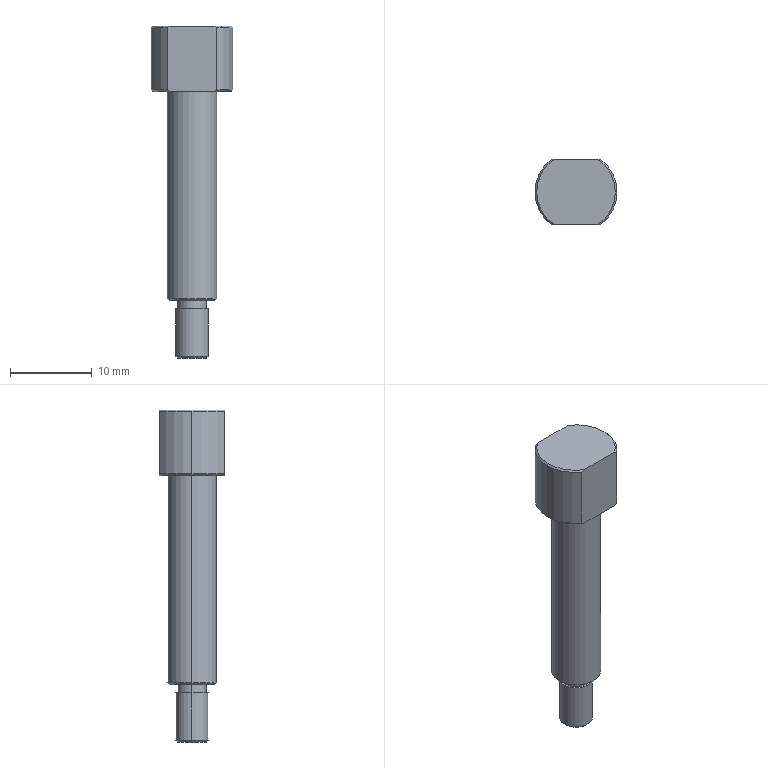Part | SolidWorks | features ICE 4, Chamfer 3, Extrusion 1 | 1 solid | 26 faces | box 10 x 8 x 40.5 mm | volume 1368 mm3 | cone 10 | cylinder 9 | plane 7 | commonest cylinder face diameters 10 x3 3.5 x2 4 x2 6 x2
STEP:
#1=CARTESIAN_POINT('',(2.,0.,-19.55));
#2=VERTEX_POINT('',#1);
#3=CARTESIAN_POINT('',(-2.,0.,-19.55));
#4=VERTEX_POINT('',#3);
#5=CARTESIAN_POINT('',(0.,0.,-19.55));
#6=DIRECTION('',(0.,0.,1.));
#7=DIRECTION('',(-1.,0.,0.));
#8=AXIS2_PLACEMENT_3D('',#5,#6,#7);
#9=CIRCLE('',#8,2.);
#10=EDGE_CURVE('',#2,#4,#9,.T.);
#11=ORIENTED_EDGE('',*,*,#10,.T.);
#12=CARTESIAN_POINT('',(-2.,0.,-13.75));
#13=VERTEX_POINT('',#12);
#14=CARTESIAN_POINT('',(-2.,0.,-19.75));
#15=DIRECTION('',(0.,0.,1.));
#16=VECTOR('',#15,1000.);
#17=LINE('',#14,#16);
#18=EDGE_CURVE('',#4,#13,#17,.T.);
#19=ORIENTED_EDGE('',*,*,#18,.T.);
#20=CARTESIAN_POINT('',(2.,0.,-13.75));
#21=VERTEX_POINT('',#20);
#22=CARTESIAN_POINT('',(0.,0.,-13.75));
#23=DIRECTION('',(0.,0.,-1.));
#24=DIRECTION('',(-1.,0.,0.));
#25=AXIS2_PLACEMENT_3D('',#22,#23,#24);
#26=CIRCLE('',#25,2.);
#27=EDGE_CURVE('',#13,#21,#26,.T.);
#28=ORIENTED_EDGE('',*,*,#27,.T.);
#29=CARTESIAN_POINT('',(2.,0.,-19.75));
#30=DIRECTION('',(0.,0.,1.));
#31=VECTOR('',#30,1000.);
#32=LINE('',#29,#31);
#33=EDGE_CURVE('',#2,#21,#32,.T.);
#34=ORIENTED_EDGE('',*,*,#33,.F.);
#35=EDGE_LOOP('',(#11,#19,#28,#34));
#36=FACE_OUTER_BOUND('',#35,.T.);
#37=CARTESIAN_POINT('',(0.,0.,-19.75));
#38=DIRECTION('',(0.,0.,1.));
#39=DIRECTION('',(1.,0.,0.));
#40=AXIS2_PLACEMENT_3D('',#37,#38,#39);
#41=CYLINDRICAL_SURFACE('',#40,2.);
#42=ADVANCED_FACE('',(#36),#41,.T.);
#43=CARTESIAN_POINT('',(-1.8,0.,-19.75));
#44=VERTEX_POINT('',#43);
#45=CARTESIAN_POINT('',(1.8,0.,-19.75));
#46=VERTEX_POINT('',#45);
#47=CARTESIAN_POINT('',(0.,0.,-19.75));
#48=DIRECTION('',(0.,0.,-1.));
#49=DIRECTION('',(-1.,0.,0.));
#50=AXIS2_PLACEMENT_3D('',#47,#48,#49);
#51=CIRCLE('',#50,1.8);
#52=EDGE_CURVE('',#44,#46,#51,.T.);
#53=ORIENTED_EDGE('',*,*,#52,.F.);
#54=CARTESIAN_POINT('',(-1.8,0.,-19.75));
#55=DIRECTION('',(-0.7071,0.,0.7071));
#56=VECTOR('',#55,1000.);
#57=LINE('',#54,#56);
#58=EDGE_CURVE('',#44,#4,#57,.T.);
#59=ORIENTED_EDGE('',*,*,#58,.T.);
#60=ORIENTED_EDGE('',*,*,#10,.F.);
#61=CARTESIAN_POINT('',(1.8,0.,-19.75));
#62=DIRECTION('',(0.7071,0.,0.7071));
#63=VECTOR('',#62,1000.);
#64=LINE('',#61,#63);
#65=EDGE_CURVE('',#46,#2,#64,.T.);
#66=ORIENTED_EDGE('',*,*,#65,.F.);
#67=EDGE_LOOP('',(#53,#59,#60,#66));
#68=FACE_OUTER_BOUND('',#67,.T.);
#69=CARTESIAN_POINT('',(0.,0.,-19.75));
#70=DIRECTION('',(0.,0.,1.));
#71=DIRECTION('',(1.,0.,0.));
#72=AXIS2_PLACEMENT_3D('',#69,#70,#71);
#73=CONICAL_SURFACE('',#72,1.8,0.7854);
#74=ADVANCED_FACE('',(#68),#73,.T.);
#75=CARTESIAN_POINT('',(-1.75,0.,-13.75));
#76=VERTEX_POINT('',#75);
#77=CARTESIAN_POINT('',(1.75,0.,-13.75));
#78=VERTEX_POINT('',#77);
#79=CARTESIAN_POINT('',(0.,0.,-13.75));
#80=DIRECTION('',(0.,0.,-1.));
#81=DIRECTION('',(-1.,0.,0.));
#82=AXIS2_PLACEMENT_3D('',#79,#80,#81);
#83=CIRCLE('',#82,1.75);
#84=EDGE_CURVE('',#76,#78,#83,.T.);
#85=ORIENTED_EDGE('',*,*,#84,.F.);
#86=CARTESIAN_POINT('',(-1.75,0.,-12.75));
#87=VERTEX_POINT('',#86);
#88=CARTESIAN_POINT('',(-1.75,0.,-13.75));
#89=DIRECTION('',(0.,0.,1.));
#90=VECTOR('',#89,1000.);
#91=LINE('',#88,#90);
#92=EDGE_CURVE('',#76,#87,#91,.T.);
#93=ORIENTED_EDGE('',*,*,#92,.T.);
#94=CARTESIAN_POINT('',(1.75,0.,-12.75));
#95=VERTEX_POINT('',#94);
#96=CARTESIAN_POINT('',(0.,0.,-12.75));
#97=DIRECTION('',(0.,0.,-1.));
#98=DIRECTION('',(-1.,0.,0.));
#99=AXIS2_PLACEMENT_3D('',#96,#97,#98);
#100=CIRCLE('',#99,1.75);
#101=EDGE_CURVE('',#87,#95,#100,.T.);
#102=ORIENTED_EDGE('',*,*,#101,.T.);
#103=CARTESIAN_POINT('',(1.75,0.,-13.75));
#104=DIRECTION('',(0.,0.,1.));
#105=VECTOR('',#104,1000.);
#106=LINE('',#103,#105);
#107=EDGE_CURVE('',#78,#95,#106,.T.);
#108=ORIENTED_EDGE('',*,*,#107,.F.);
#109=EDGE_LOOP('',(#85,#93,#102,#108));
#110=FACE_OUTER_BOUND('',#109,.T.);
#111=CARTESIAN_POINT('',(0.,0.,-13.75));
#112=DIRECTION('',(0.,0.,1.));
#113=DIRECTION('',(1.,0.,0.));
#114=AXIS2_PLACEMENT_3D('',#111,#112,#113);
#115=CYLINDRICAL_SURFACE('',#114,1.75);
#116=ADVANCED_FACE('',(#110),#115,.T.);
#117=CARTESIAN_POINT('',(4.8,0.,12.75));
#118=VERTEX_POINT('',#117);
#119=CARTESIAN_POINT('',(2.653,-4.,12.75));
#120=VERTEX_POINT('',#119);
#121=CARTESIAN_POINT('',(0.,0.,12.75));
#122=DIRECTION('',(0.,0.,-1.));
#123=DIRECTION('',(1.,0.,0.));
#124=AXIS2_PLACEMENT_3D('',#121,#122,#123);
#125=CIRCLE('',#124,4.8);
#126=EDGE_CURVE('',#118,#120,#125,.T.);
#127=ORIENTED_EDGE('',*,*,#126,.F.);
#128=CARTESIAN_POINT('',(5.,0.,12.95));
#129=VERTEX_POINT('',#128);
#130=CARTESIAN_POINT('',(5.,0.,12.95));
#131=DIRECTION('',(0.7071,0.,0.7071));
#132=VECTOR('',#131,1000.);
#133=LINE('',#130,#132);
#134=EDGE_CURVE('',#118,#129,#133,.T.);
#135=ORIENTED_EDGE('',*,*,#134,.T.);
#136=CARTESIAN_POINT('',(3.,-4.,12.95));
#137=VERTEX_POINT('',#136);
#138=CARTESIAN_POINT('',(0.,0.,12.95));
#139=DIRECTION('',(0.,0.,1.));
#140=DIRECTION('',(1.,0.,0.));
#141=AXIS2_PLACEMENT_3D('',#138,#139,#140);
#142=CIRCLE('',#141,5.);
#143=EDGE_CURVE('',#137,#129,#142,.T.);
#144=ORIENTED_EDGE('',*,*,#143,.F.);
#145=CARTESIAN_POINT('',(2.653,-4.,12.75));
#146=CARTESIAN_POINT('',(2.77,-4.,12.815));
#147=CARTESIAN_POINT('',(2.886,-4.,12.881));
#148=CARTESIAN_POINT('',(3.,-4.,12.95));
#149=B_SPLINE_CURVE_WITH_KNOTS('',3,(#145,#146,#147,#148),.UNSPECIFIED.,.F.,.F.,(4,4),(0.01544,0.01584),.UNSPECIFIED.);
#150=EDGE_CURVE('',#120,#137,#149,.T.);
#151=ORIENTED_EDGE('',*,*,#150,.F.);
#152=EDGE_LOOP('',(#127,#135,#144,#151));
#153=FACE_OUTER_BOUND('',#152,.T.);
#154=CARTESIAN_POINT('',(0.,0.,12.95));
#155=DIRECTION('',(0.,0.,1.));
#156=DIRECTION('',(1.,0.,0.));
#157=AXIS2_PLACEMENT_3D('',#154,#155,#156);
#158=CONICAL_SURFACE('',#157,5.,0.7854);
#159=ADVANCED_FACE('',(#153),#158,.T.);
#160=CARTESIAN_POINT('',(-4.8,0.,20.75));
#161=VERTEX_POINT('',#160);
#162=CARTESIAN_POINT('',(-2.653,-4.,20.75));
#163=VERTEX_POINT('',#162);
#164=CARTESIAN_POINT('',(0.,0.,20.75));
#165=DIRECTION('',(0.,0.,1.));
#166=DIRECTION('',(1.,0.,0.));
#167=AXIS2_PLACEMENT_3D('',#164,#165,#166);
#168=CIRCLE('',#167,4.8);
#169=EDGE_CURVE('',#161,#163,#168,.T.);
#170=ORIENTED_EDGE('',*,*,#169,.F.);
#171=CARTESIAN_POINT('',(-5.,0.,20.55));
#172=VERTEX_POINT('',#171);
#173=CARTESIAN_POINT('',(-4.8,0.,20.75));
#174=DIRECTION('',(-0.7071,0.,-0.7071));
#175=VECTOR('',#174,1000.);
#176=LINE('',#173,#175);
#177=EDGE_CURVE('',#161,#172,#176,.T.);
#178=ORIENTED_EDGE('',*,*,#177,.T.);
#179=CARTESIAN_POINT('',(-3.,-4.,20.55));
#180=VERTEX_POINT('',#179);
#181=CARTESIAN_POINT('',(0.,0.,20.55));
#182=DIRECTION('',(0.,0.,-1.));
#183=DIRECTION('',(1.,0.,0.));
#184=AXIS2_PLACEMENT_3D('',#181,#182,#183);
#185=CIRCLE('',#184,5.);
#186=EDGE_CURVE('',#180,#172,#185,.T.);
#187=ORIENTED_EDGE('',*,*,#186,.F.);
#188=CARTESIAN_POINT('',(-2.653,-4.,20.75));
#189=CARTESIAN_POINT('',(-2.77,-4.,20.685));
#190=CARTESIAN_POINT('',(-2.886,-4.,20.619));
#191=CARTESIAN_POINT('',(-3.,-4.,20.55));
#192=B_SPLINE_CURVE_WITH_KNOTS('',3,(#188,#189,#190,#191),.UNSPECIFIED.,.F.,.F.,(4,4),(0.01544,0.01584),.UNSPECIFIED.);
#193=EDGE_CURVE('',#163,#180,#192,.T.);
#194=ORIENTED_EDGE('',*,*,#193,.F.);
#195=EDGE_LOOP('',(#170,#178,#187,#194));
#196=FACE_OUTER_BOUND('',#195,.T.);
#197=CARTESIAN_POINT('',(0.,0.,20.75));
#198=DIRECTION('',(0.,0.,-1.));
#199=DIRECTION('',(-1.,0.,0.));
#200=AXIS2_PLACEMENT_3D('',#197,#198,#199);
#201=CONICAL_SURFACE('',#200,4.8,0.7854);
#202=ADVANCED_FACE('',(#196),#201,.T.);
#203=ORIENTED_EDGE('',*,*,#186,.T.);
#204=CARTESIAN_POINT('',(-5.,0.,12.95));
#205=VERTEX_POINT('',#204);
#206=CARTESIAN_POINT('',(-5.,0.,20.75));
#207=DIRECTION('',(0.,0.,-1.));
#208=VECTOR('',#207,1000.);
#209=LINE('',#206,#208);
#210=EDGE_CURVE('',#172,#205,#209,.T.);
#211=ORIENTED_EDGE('',*,*,#210,.T.);
#212=CARTESIAN_POINT('',(-3.,-4.,12.95));
#213=VERTEX_POINT('',#212);
#214=CARTESIAN_POINT('',(0.,0.,12.95));
#215=DIRECTION('',(0.,0.,1.));
#216=DIRECTION('',(1.,0.,0.));
#217=AXIS2_PLACEMENT_3D('',#214,#215,#216);
#218=CIRCLE('',#217,5.);
#219=EDGE_CURVE('',#205,#213,#218,.T.);
#220=ORIENTED_EDGE('',*,*,#219,.T.);
#221=CARTESIAN_POINT('',(-3.,-4.,20.75));
#222=DIRECTION('',(0.,0.,1.));
#223=VECTOR('',#222,1000.);
#224=LINE('',#221,#223);
#225=EDGE_CURVE('',#213,#180,#224,.T.);
#226=ORIENTED_EDGE('',*,*,#225,.T.);
#227=EDGE_LOOP('',(#203,#211,#220,#226));
#228=FACE_OUTER_BOUND('',#227,.T.);
#229=CARTESIAN_POINT('',(0.,0.,20.75));
#230=DIRECTION('',(0.,0.,-1.));
#231=DIRECTION('',(-1.,0.,0.));
#232=AXIS2_PLACEMENT_3D('',#229,#230,#231);
#233=CYLINDRICAL_SURFACE('',#232,5.);
#234=ADVANCED_FACE('',(#228),#233,.T.);
#235=CARTESIAN_POINT('',(-2.8,0.,-12.75));
#236=VERTEX_POINT('',#235);
#237=CARTESIAN_POINT('',(2.8,0.,-12.75));
#238=VERTEX_POINT('',#237);
#239=CARTESIAN_POINT('',(0.,0.,-12.75));
#240=DIRECTION('',(0.,0.,-1.));
#241=DIRECTION('',(1.,0.,0.));
#242=AXIS2_PLACEMENT_3D('',#239,#240,#241);
#243=CIRCLE('',#242,2.8);
#244=EDGE_CURVE('',#236,#238,#243,.T.);
#245=ORIENTED_EDGE('',*,*,#244,.F.);
#246=CARTESIAN_POINT('',(-3.,0.,-12.55));
#247=VERTEX_POINT('',#246);
#248=CARTESIAN_POINT('',(-3.,0.,-12.55));
#249=DIRECTION('',(-0.7071,0.,0.7071));
#250=VECTOR('',#249,1000.);
#251=LINE('',#248,#250);
#252=EDGE_CURVE('',#236,#247,#251,.T.);
#253=ORIENTED_EDGE('',*,*,#252,.T.);
#254=CARTESIAN_POINT('',(3.,0.,-12.55));
#255=VERTEX_POINT('',#254);
#256=CARTESIAN_POINT('',(0.,0.,-12.55));
#257=DIRECTION('',(0.,0.,1.));
#258=DIRECTION('',(1.,0.,0.));
#259=AXIS2_PLACEMENT_3D('',#256,#257,#258);
#260=CIRCLE('',#259,3.);
#261=EDGE_CURVE('',#255,#247,#260,.T.);
#262=ORIENTED_EDGE('',*,*,#261,.F.);
#263=CARTESIAN_POINT('',(3.,0.,-12.55));
#264=DIRECTION('',(0.7071,0.,0.7071));
#265=VECTOR('',#264,1000.);
#266=LINE('',#263,#265);
#267=EDGE_CURVE('',#238,#255,#266,.T.);
#268=ORIENTED_EDGE('',*,*,#267,.F.);
#269=EDGE_LOOP('',(#245,#253,#262,#268));
#270=FACE_OUTER_BOUND('',#269,.T.);
#271=CARTESIAN_POINT('',(0.,0.,-12.55));
#272=DIRECTION('',(0.,0.,1.));
#273=DIRECTION('',(1.,0.,0.));
#274=AXIS2_PLACEMENT_3D('',#271,#272,#273);
#275=CONICAL_SURFACE('',#274,3.,0.7854);
#276=ADVANCED_FACE('',(#270),#275,.T.);
#277=CARTESIAN_POINT('',(3.,0.,12.75));
#278=VERTEX_POINT('',#277);
#279=CARTESIAN_POINT('',(-3.,0.,12.75));
#280=VERTEX_POINT('',#279);
#281=CARTESIAN_POINT('',(0.,0.,12.75));
#282=DIRECTION('',(0.,0.,1.));
#283=DIRECTION('',(1.,0.,0.));
#284=AXIS2_PLACEMENT_3D('',#281,#282,#283);
#285=CIRCLE('',#284,3.);
#286=EDGE_CURVE('',#278,#280,#285,.T.);
#287=ORIENTED_EDGE('',*,*,#286,.F.);
#288=CARTESIAN_POINT('',(3.,0.,12.75));
#289=DIRECTION('',(0.,0.,-1.));
#290=VECTOR('',#289,1000.);
#291=LINE('',#288,#290);
#292=EDGE_CURVE('',#278,#255,#291,.T.);
#293=ORIENTED_EDGE('',*,*,#292,.T.);
#294=ORIENTED_EDGE('',*,*,#261,.T.);
#295=CARTESIAN_POINT('',(-3.,0.,12.75));
#296=DIRECTION('',(0.,0.,-1.));
#297=VECTOR('',#296,1000.);
#298=LINE('',#295,#297);
#299=EDGE_CURVE('',#280,#247,#298,.T.);
#300=ORIENTED_EDGE('',*,*,#299,.F.);
#301=EDGE_LOOP('',(#287,#293,#294,#300));
#302=FACE_OUTER_BOUND('',#301,.T.);
#303=CARTESIAN_POINT('',(0.,0.,12.75));
#304=DIRECTION('',(0.,0.,-1.));
#305=DIRECTION('',(-1.,0.,0.));
#306=AXIS2_PLACEMENT_3D('',#303,#304,#305);
#307=CYLINDRICAL_SURFACE('',#306,3.);
#308=ADVANCED_FACE('',(#302),#307,.T.);
#309=CARTESIAN_POINT('',(3.,4.,20.55));
#310=VERTEX_POINT('',#309);
#311=CARTESIAN_POINT('',(3.,-4.,20.55));
#312=VERTEX_POINT('',#311);
#313=CARTESIAN_POINT('',(0.,0.,20.55));
#314=DIRECTION('',(0.,0.,-1.));
#315=DIRECTION('',(1.,0.,0.));
#316=AXIS2_PLACEMENT_3D('',#313,#314,#315);
#317=CIRCLE('',#316,5.);
#318=EDGE_CURVE('',#310,#312,#317,.T.);
#319=ORIENTED_EDGE('',*,*,#318,.T.);
#320=CARTESIAN_POINT('',(3.,-4.,20.75));
#321=DIRECTION('',(0.,0.,-1.));
#322=VECTOR('',#321,1000.);
#323=LINE('',#320,#322);
#324=EDGE_CURVE('',#312,#137,#323,.T.);
#325=ORIENTED_EDGE('',*,*,#324,.T.);
#326=ORIENTED_EDGE('',*,*,#143,.T.);
#327=CARTESIAN_POINT('',(3.,4.,12.95));
#328=VERTEX_POINT('',#327);
#329=CARTESIAN_POINT('',(0.,0.,12.95));
#330=DIRECTION('',(0.,0.,1.));
#331=DIRECTION('',(1.,0.,0.));
#332=AXIS2_PLACEMENT_3D('',#329,#330,#331);
#333=CIRCLE('',#332,5.);
#334=EDGE_CURVE('',#129,#328,#333,.T.);
#335=ORIENTED_EDGE('',*,*,#334,.T.);
#336=CARTESIAN_POINT('',(3.,4.,20.75));
#337=DIRECTION('',(0.,0.,1.));
#338=VECTOR('',#337,1000.);
#339=LINE('',#336,#338);
#340=EDGE_CURVE('',#328,#310,#339,.T.);
#341=ORIENTED_EDGE('',*,*,#340,.T.);
#342=EDGE_LOOP('',(#319,#325,#326,#335,#341));
#343=FACE_OUTER_BOUND('',#342,.T.);
#344=CARTESIAN_POINT('',(0.,0.,20.75));
#345=DIRECTION('',(0.,0.,-1.));
#346=DIRECTION('',(-1.,0.,0.));
#347=AXIS2_PLACEMENT_3D('',#344,#345,#346);
#348=CYLINDRICAL_SURFACE('',#347,5.);
#349=ADVANCED_FACE('',(#343),#348,.T.);
#350=CARTESIAN_POINT('',(2.653,-4.,20.75));
#351=VERTEX_POINT('',#350);
#352=CARTESIAN_POINT('',(3.,-4.,20.55));
#353=CARTESIAN_POINT('',(2.885,-4.,20.619));
#354=CARTESIAN_POINT('',(2.77,-4.,20.686));
#355=CARTESIAN_POINT('',(2.653,-4.,20.75));
#356=B_SPLINE_CURVE_WITH_KNOTS('',3,(#352,#353,#354,#355),.UNSPECIFIED.,.F.,.F.,(4,4),(0.009425,0.009825),.UNSPECIFIED.);
#357=EDGE_CURVE('',#312,#351,#356,.T.);
#358=ORIENTED_EDGE('',*,*,#357,.F.);
#359=ORIENTED_EDGE('',*,*,#318,.F.);
#360=CARTESIAN_POINT('',(2.653,4.,20.75));
#361=VERTEX_POINT('',#360);
#362=CARTESIAN_POINT('',(2.653,4.,20.75));
#363=CARTESIAN_POINT('',(2.77,4.,20.685));
#364=CARTESIAN_POINT('',(2.886,4.,20.619));
#365=CARTESIAN_POINT('',(3.,4.,20.55));
#366=B_SPLINE_CURVE_WITH_KNOTS('',3,(#362,#363,#364,#365),.UNSPECIFIED.,.F.,.F.,(4,4),(0.01544,0.01584),.UNSPECIFIED.);
#367=EDGE_CURVE('',#361,#310,#366,.T.);
#368=ORIENTED_EDGE('',*,*,#367,.F.);
#369=CARTESIAN_POINT('',(0.,0.,20.75));
#370=DIRECTION('',(0.,0.,1.));
#371=DIRECTION('',(1.,0.,0.));
#372=AXIS2_PLACEMENT_3D('',#369,#370,#371);
#373=CIRCLE('',#372,4.8);
#374=EDGE_CURVE('',#351,#361,#373,.T.);
#375=ORIENTED_EDGE('',*,*,#374,.F.);
#376=EDGE_LOOP('',(#358,#359,#368,#375));
#377=FACE_OUTER_BOUND('',#376,.T.);
#378=CARTESIAN_POINT('',(0.,0.,20.75));
#379=DIRECTION('',(0.,0.,-1.));
#380=DIRECTION('',(-1.,0.,0.));
#381=AXIS2_PLACEMENT_3D('',#378,#379,#380);
#382=CONICAL_SURFACE('',#381,4.8,0.7854);
#383=ADVANCED_FACE('',(#377),#382,.T.);
#384=CARTESIAN_POINT('',(-2.653,-4.,12.75));
#385=VERTEX_POINT('',#384);
#386=CARTESIAN_POINT('',(-3.,-4.,12.95));
#387=CARTESIAN_POINT('',(-2.885,-4.,12.881));
#388=CARTESIAN_POINT('',(-2.77,-4.,12.814));
#389=CARTESIAN_POINT('',(-2.653,-4.,12.75));
#390=B_SPLINE_CURVE_WITH_KNOTS('',3,(#386,#387,#388,#389),.UNSPECIFIED.,.F.,.F.,(4,4),(0.009425,0.009825),.UNSPECIFIED.);
#391=EDGE_CURVE('',#213,#385,#390,.T.);
#392=ORIENTED_EDGE('',*,*,#391,.F.);
#393=ORIENTED_EDGE('',*,*,#219,.F.);
#394=CARTESIAN_POINT('',(-3.,4.,12.95));
#395=VERTEX_POINT('',#394);
#396=CARTESIAN_POINT('',(0.,0.,12.95));
#397=DIRECTION('',(0.,0.,1.));
#398=DIRECTION('',(1.,0.,0.));
#399=AXIS2_PLACEMENT_3D('',#396,#397,#398);
#400=CIRCLE('',#399,5.);
#401=EDGE_CURVE('',#395,#205,#400,.T.);
#402=ORIENTED_EDGE('',*,*,#401,.F.);
#403=CARTESIAN_POINT('',(-2.653,4.,12.75));
#404=VERTEX_POINT('',#403);
#405=CARTESIAN_POINT('',(-2.653,4.,12.75));
#406=CARTESIAN_POINT('',(-2.77,4.,12.815));
#407=CARTESIAN_POINT('',(-2.886,4.,12.881));
#408=CARTESIAN_POINT('',(-3.,4.,12.95));
#409=B_SPLINE_CURVE_WITH_KNOTS('',3,(#405,#406,#407,#408),.UNSPECIFIED.,.F.,.F.,(4,4),(0.01544,0.01584),.UNSPECIFIED.);
#410=EDGE_CURVE('',#404,#395,#409,.T.);
#411=ORIENTED_EDGE('',*,*,#410,.F.);
#412=CARTESIAN_POINT('',(0.,0.,12.75));
#413=DIRECTION('',(0.,0.,-1.));
#414=DIRECTION('',(1.,0.,0.));
#415=AXIS2_PLACEMENT_3D('',#412,#413,#414);
#416=CIRCLE('',#415,4.8);
#417=EDGE_CURVE('',#385,#404,#416,.T.);
#418=ORIENTED_EDGE('',*,*,#417,.F.);
#419=EDGE_LOOP('',(#392,#393,#402,#411,#418));
#420=FACE_OUTER_BOUND('',#419,.T.);
#421=CARTESIAN_POINT('',(0.,0.,12.95));
#422=DIRECTION('',(0.,0.,1.));
#423=DIRECTION('',(1.,0.,0.));
#424=AXIS2_PLACEMENT_3D('',#421,#422,#423);
#425=CONICAL_SURFACE('',#424,5.,0.7854);
#426=ADVANCED_FACE('',(#420),#425,.T.);
#427=CARTESIAN_POINT('',(0.,0.,-12.75));
#428=DIRECTION('',(0.,0.,-1.));
#429=DIRECTION('',(1.,0.,0.));
#430=AXIS2_PLACEMENT_3D('',#427,#428,#429);
#431=CIRCLE('',#430,2.8);
#432=EDGE_CURVE('',#238,#236,#431,.T.);
#433=ORIENTED_EDGE('',*,*,#432,.T.);
#434=ORIENTED_EDGE('',*,*,#244,.T.);
#435=EDGE_LOOP('',(#433,#434));
#436=FACE_OUTER_BOUND('',#435,.T.);
#437=CARTESIAN_POINT('',(0.,0.,-12.75));
#438=DIRECTION('',(0.,0.,-1.));
#439=DIRECTION('',(-1.,0.,0.));
#440=AXIS2_PLACEMENT_3D('',#437,#438,#439);
#441=CIRCLE('',#440,1.75);
#442=EDGE_CURVE('',#95,#87,#441,.T.);
#443=ORIENTED_EDGE('',*,*,#442,.F.);
#444=ORIENTED_EDGE('',*,*,#101,.F.);
#445=EDGE_LOOP('',(#443,#444));
#446=FACE_BOUND('',#445,.T.);
#447=CARTESIAN_POINT('',(0.,0.,-12.75));
#448=DIRECTION('',(0.,0.,1.));
#449=DIRECTION('',(1.,0.,0.));
#450=AXIS2_PLACEMENT_3D('',#447,#448,#449);
#451=PLANE('',#450);
#452=ADVANCED_FACE('',(#436,#446),#451,.F.);
#453=ORIENTED_EDGE('',*,*,#292,.F.);
#454=CARTESIAN_POINT('',(0.,0.,12.75));
#455=DIRECTION('',(0.,0.,1.));
#456=DIRECTION('',(1.,0.,0.));
#457=AXIS2_PLACEMENT_3D('',#454,#455,#456);
#458=CIRCLE('',#457,3.);
#459=EDGE_CURVE('',#280,#278,#458,.T.);
#460=ORIENTED_EDGE('',*,*,#459,.F.);
#461=ORIENTED_EDGE('',*,*,#299,.T.);
#462=CARTESIAN_POINT('',(0.,0.,-12.55));
#463=DIRECTION('',(0.,0.,1.));
#464=DIRECTION('',(1.,0.,0.));
#465=AXIS2_PLACEMENT_3D('',#462,#463,#464);
#466=CIRCLE('',#465,3.);
#467=EDGE_CURVE('',#247,#255,#466,.T.);
#468=ORIENTED_EDGE('',*,*,#467,.T.);
#469=EDGE_LOOP('',(#453,#460,#461,#468));
#470=FACE_OUTER_BOUND('',#469,.T.);
#471=CARTESIAN_POINT('',(0.,0.,12.75));
#472=DIRECTION('',(0.,0.,-1.));
#473=DIRECTION('',(-1.,0.,0.));
#474=AXIS2_PLACEMENT_3D('',#471,#472,#473);
#475=CYLINDRICAL_SURFACE('',#474,3.);
#476=ADVANCED_FACE('',(#470),#475,.T.);
#477=ORIENTED_EDGE('',*,*,#252,.F.);
#478=ORIENTED_EDGE('',*,*,#432,.F.);
#479=ORIENTED_EDGE('',*,*,#267,.T.);
#480=ORIENTED_EDGE('',*,*,#467,.F.);
#481=EDGE_LOOP('',(#477,#478,#479,#480));
#482=FACE_OUTER_BOUND('',#481,.T.);
#483=CARTESIAN_POINT('',(0.,0.,-12.55));
#484=DIRECTION('',(0.,0.,1.));
#485=DIRECTION('',(1.,0.,0.));
#486=AXIS2_PLACEMENT_3D('',#483,#484,#485);
#487=CONICAL_SURFACE('',#486,3.,0.7854);
#488=ADVANCED_FACE('',(#482),#487,.T.);
#489=CARTESIAN_POINT('',(2.653,4.,12.75));
#490=VERTEX_POINT('',#489);
#491=CARTESIAN_POINT('',(0.,0.,12.75));
#492=DIRECTION('',(0.,0.,-1.));
#493=DIRECTION('',(1.,0.,0.));
#494=AXIS2_PLACEMENT_3D('',#491,#492,#493);
#495=CIRCLE('',#494,4.8);
#496=EDGE_CURVE('',#490,#118,#495,.T.);
#497=ORIENTED_EDGE('',*,*,#496,.T.);
#498=ORIENTED_EDGE('',*,*,#126,.T.);
#499=CARTESIAN_POINT('',(18.476,-4.,12.75));
#500=DIRECTION('',(1.,0.,0.));
#501=VECTOR('',#500,1000.);
#502=LINE('',#499,#501);
#503=EDGE_CURVE('',#385,#120,#502,.T.);
#504=ORIENTED_EDGE('',*,*,#503,.F.);
#505=ORIENTED_EDGE('',*,*,#417,.T.);
#506=CARTESIAN_POINT('',(-15.736,4.,12.75));
#507=DIRECTION('',(-1.,0.,0.));
#508=VECTOR('',#507,1000.);
#509=LINE('',#506,#508);
#510=EDGE_CURVE('',#490,#404,#509,.T.);
#511=ORIENTED_EDGE('',*,*,#510,.F.);
#512=EDGE_LOOP('',(#497,#498,#504,#505,#511));
#513=FACE_OUTER_BOUND('',#512,.T.);
#514=ORIENTED_EDGE('',*,*,#459,.T.);
#515=ORIENTED_EDGE('',*,*,#286,.T.);
#516=EDGE_LOOP('',(#514,#515));
#517=FACE_BOUND('',#516,.T.);
#518=CARTESIAN_POINT('',(0.,0.,12.75));
#519=DIRECTION('',(0.,0.,1.));
#520=DIRECTION('',(1.,0.,0.));
#521=AXIS2_PLACEMENT_3D('',#518,#519,#520);
#522=PLANE('',#521);
#523=ADVANCED_FACE('',(#513,#517),#522,.F.);
#524=ORIENTED_EDGE('',*,*,#210,.F.);
#525=CARTESIAN_POINT('',(-3.,4.,20.55));
#526=VERTEX_POINT('',#525);
#527=CARTESIAN_POINT('',(0.,0.,20.55));
#528=DIRECTION('',(0.,0.,-1.));
#529=DIRECTION('',(1.,0.,0.));
#530=AXIS2_PLACEMENT_3D('',#527,#528,#529);
#531=CIRCLE('',#530,5.);
#532=EDGE_CURVE('',#172,#526,#531,.T.);
#533=ORIENTED_EDGE('',*,*,#532,.T.);
#534=CARTESIAN_POINT('',(-3.,4.,20.75));
#535=DIRECTION('',(0.,0.,-1.));
#536=VECTOR('',#535,1000.);
#537=LINE('',#534,#536);
#538=EDGE_CURVE('',#526,#395,#537,.T.);
#539=ORIENTED_EDGE('',*,*,#538,.T.);
#540=ORIENTED_EDGE('',*,*,#401,.T.);
#541=EDGE_LOOP('',(#524,#533,#539,#540));
#542=FACE_OUTER_BOUND('',#541,.T.);
#543=CARTESIAN_POINT('',(0.,0.,20.75));
#544=DIRECTION('',(0.,0.,-1.));
#545=DIRECTION('',(-1.,0.,0.));
#546=AXIS2_PLACEMENT_3D('',#543,#544,#545);
#547=CYLINDRICAL_SURFACE('',#546,5.);
#548=ADVANCED_FACE('',(#542),#547,.T.);
#549=CARTESIAN_POINT('',(18.476,-4.,20.75));
#550=DIRECTION('',(-1.,0.,0.));
#551=VECTOR('',#550,1000.);
#552=LINE('',#549,#551);
#553=EDGE_CURVE('',#351,#163,#552,.T.);
#554=ORIENTED_EDGE('',*,*,#553,.F.);
#555=ORIENTED_EDGE('',*,*,#374,.T.);
#556=CARTESIAN_POINT('',(-2.653,4.,20.75));
#557=VERTEX_POINT('',#556);
#558=CARTESIAN_POINT('',(-15.736,4.,20.75));
#559=DIRECTION('',(1.,0.,0.));
#560=VECTOR('',#559,1000.);
#561=LINE('',#558,#560);
#562=EDGE_CURVE('',#557,#361,#561,.T.);
#563=ORIENTED_EDGE('',*,*,#562,.F.);
#564=CARTESIAN_POINT('',(0.,0.,20.75));
#565=DIRECTION('',(0.,0.,1.));
#566=DIRECTION('',(1.,0.,0.));
#567=AXIS2_PLACEMENT_3D('',#564,#565,#566);
#568=CIRCLE('',#567,4.8);
#569=EDGE_CURVE('',#557,#161,#568,.T.);
#570=ORIENTED_EDGE('',*,*,#569,.T.);
#571=ORIENTED_EDGE('',*,*,#169,.T.);
#572=EDGE_LOOP('',(#554,#555,#563,#570,#571));
#573=FACE_OUTER_BOUND('',#572,.T.);
#574=CARTESIAN_POINT('',(0.,0.,20.75));
#575=DIRECTION('',(0.,0.,1.));
#576=DIRECTION('',(1.,0.,0.));
#577=AXIS2_PLACEMENT_3D('',#574,#575,#576);
#578=PLANE('',#577);
#579=ADVANCED_FACE('',(#573),#578,.T.);
#580=ORIENTED_EDGE('',*,*,#177,.F.);
#581=ORIENTED_EDGE('',*,*,#569,.F.);
#582=CARTESIAN_POINT('',(-3.,4.,20.55));
#583=CARTESIAN_POINT('',(-2.885,4.,20.619));
#584=CARTESIAN_POINT('',(-2.77,4.,20.686));
#585=CARTESIAN_POINT('',(-2.653,4.,20.75));
#586=B_SPLINE_CURVE_WITH_KNOTS('',3,(#582,#583,#584,#585),.UNSPECIFIED.,.F.,.F.,(4,4),(0.009425,0.009825),.UNSPECIFIED.);
#587=EDGE_CURVE('',#526,#557,#586,.T.);
#588=ORIENTED_EDGE('',*,*,#587,.F.);
#589=ORIENTED_EDGE('',*,*,#532,.F.);
#590=EDGE_LOOP('',(#580,#581,#588,#589));
#591=FACE_OUTER_BOUND('',#590,.T.);
#592=CARTESIAN_POINT('',(0.,0.,20.75));
#593=DIRECTION('',(0.,0.,-1.));
#594=DIRECTION('',(-1.,0.,0.));
#595=AXIS2_PLACEMENT_3D('',#592,#593,#594);
#596=CONICAL_SURFACE('',#595,4.8,0.7854);
#597=ADVANCED_FACE('',(#591),#596,.T.);
#598=ORIENTED_EDGE('',*,*,#134,.F.);
#599=ORIENTED_EDGE('',*,*,#496,.F.);
#600=CARTESIAN_POINT('',(3.,4.,12.95));
#601=CARTESIAN_POINT('',(2.885,4.,12.881));
#602=CARTESIAN_POINT('',(2.77,4.,12.814));
#603=CARTESIAN_POINT('',(2.653,4.,12.75));
#604=B_SPLINE_CURVE_WITH_KNOTS('',3,(#600,#601,#602,#603),.UNSPECIFIED.,.F.,.F.,(4,4),(0.009425,0.009825),.UNSPECIFIED.);
#605=EDGE_CURVE('',#328,#490,#604,.T.);
#606=ORIENTED_EDGE('',*,*,#605,.F.);
#607=ORIENTED_EDGE('',*,*,#334,.F.);
#608=EDGE_LOOP('',(#598,#599,#606,#607));
#609=FACE_OUTER_BOUND('',#608,.T.);
#610=CARTESIAN_POINT('',(0.,0.,12.95));
#611=DIRECTION('',(0.,0.,1.));
#612=DIRECTION('',(1.,0.,0.));
#613=AXIS2_PLACEMENT_3D('',#610,#611,#612);
#614=CONICAL_SURFACE('',#613,5.,0.7854);
#615=ADVANCED_FACE('',(#609),#614,.T.);
#616=ORIENTED_EDGE('',*,*,#367,.T.);
#617=ORIENTED_EDGE('',*,*,#340,.F.);
#618=ORIENTED_EDGE('',*,*,#605,.T.);
#619=ORIENTED_EDGE('',*,*,#510,.T.);
#620=ORIENTED_EDGE('',*,*,#410,.T.);
#621=ORIENTED_EDGE('',*,*,#538,.F.);
#622=ORIENTED_EDGE('',*,*,#587,.T.);
#623=ORIENTED_EDGE('',*,*,#562,.T.);
#624=EDGE_LOOP('',(#616,#617,#618,#619,#620,#621,#622,#623));
#625=FACE_OUTER_BOUND('',#624,.T.);
#626=CARTESIAN_POINT('',(-15.736,4.,-12.601));
#627=DIRECTION('',(0.,-1.,0.));
#628=DIRECTION('',(0.,0.,-1.));
#629=AXIS2_PLACEMENT_3D('',#626,#627,#628);
#630=PLANE('',#629);
#631=ADVANCED_FACE('',(#625),#630,.F.);
#632=ORIENTED_EDGE('',*,*,#193,.T.);
#633=ORIENTED_EDGE('',*,*,#225,.F.);
#634=ORIENTED_EDGE('',*,*,#391,.T.);
#635=ORIENTED_EDGE('',*,*,#503,.T.);
#636=ORIENTED_EDGE('',*,*,#150,.T.);
#637=ORIENTED_EDGE('',*,*,#324,.F.);
#638=ORIENTED_EDGE('',*,*,#357,.T.);
#639=ORIENTED_EDGE('',*,*,#553,.T.);
#640=EDGE_LOOP('',(#632,#633,#634,#635,#636,#637,#638,#639));
#641=FACE_OUTER_BOUND('',#640,.T.);
#642=CARTESIAN_POINT('',(18.476,-4.,-12.601));
#643=DIRECTION('',(0.,1.,0.));
#644=DIRECTION('',(-1.,0.,0.));
#645=AXIS2_PLACEMENT_3D('',#642,#643,#644);
#646=PLANE('',#645);
#647=ADVANCED_FACE('',(#641),#646,.F.);
#648=CARTESIAN_POINT('',(0.,0.,-13.75));
#649=DIRECTION('',(0.,0.,-1.));
#650=DIRECTION('',(-1.,0.,0.));
#651=AXIS2_PLACEMENT_3D('',#648,#649,#650);
#652=CIRCLE('',#651,1.75);
#653=EDGE_CURVE('',#78,#76,#652,.T.);
#654=ORIENTED_EDGE('',*,*,#653,.T.);
#655=ORIENTED_EDGE('',*,*,#84,.T.);
#656=EDGE_LOOP('',(#654,#655));
#657=FACE_BOUND('',#656,.T.);
#658=CARTESIAN_POINT('',(0.,0.,-13.75));
#659=DIRECTION('',(0.,0.,-1.));
#660=DIRECTION('',(-1.,0.,0.));
#661=AXIS2_PLACEMENT_3D('',#658,#659,#660);
#662=CIRCLE('',#661,2.);
#663=EDGE_CURVE('',#21,#13,#662,.T.);
#664=ORIENTED_EDGE('',*,*,#663,.F.);
#665=ORIENTED_EDGE('',*,*,#27,.F.);
#666=EDGE_LOOP('',(#664,#665));
#667=FACE_OUTER_BOUND('',#666,.T.);
#668=CARTESIAN_POINT('',(0.,0.,-13.75));
#669=DIRECTION('',(0.,0.,-1.));
#670=DIRECTION('',(-1.,0.,0.));
#671=AXIS2_PLACEMENT_3D('',#668,#669,#670);
#672=PLANE('',#671);
#673=ADVANCED_FACE('',(#657,#667),#672,.F.);
#674=ORIENTED_EDGE('',*,*,#92,.F.);
#675=ORIENTED_EDGE('',*,*,#653,.F.);
#676=ORIENTED_EDGE('',*,*,#107,.T.);
#677=ORIENTED_EDGE('',*,*,#442,.T.);
#678=EDGE_LOOP('',(#674,#675,#676,#677));
#679=FACE_OUTER_BOUND('',#678,.T.);
#680=CARTESIAN_POINT('',(0.,0.,-13.75));
#681=DIRECTION('',(0.,0.,1.));
#682=DIRECTION('',(1.,0.,0.));
#683=AXIS2_PLACEMENT_3D('',#680,#681,#682);
#684=CYLINDRICAL_SURFACE('',#683,1.75);
#685=ADVANCED_FACE('',(#679),#684,.T.);
#686=CARTESIAN_POINT('',(0.,0.,-19.75));
#687=DIRECTION('',(0.,0.,-1.));
#688=DIRECTION('',(-1.,0.,0.));
#689=AXIS2_PLACEMENT_3D('',#686,#687,#688);
#690=CIRCLE('',#689,1.8);
#691=EDGE_CURVE('',#46,#44,#690,.T.);
#692=ORIENTED_EDGE('',*,*,#691,.T.);
#693=ORIENTED_EDGE('',*,*,#52,.T.);
#694=EDGE_LOOP('',(#692,#693));
#695=FACE_OUTER_BOUND('',#694,.T.);
#696=CARTESIAN_POINT('',(0.,0.,-19.75));
#697=DIRECTION('',(0.,0.,-1.));
#698=DIRECTION('',(-1.,0.,0.));
#699=AXIS2_PLACEMENT_3D('',#696,#697,#698);
#700=PLANE('',#699);
#701=ADVANCED_FACE('',(#695),#700,.T.);
#702=ORIENTED_EDGE('',*,*,#58,.F.);
#703=ORIENTED_EDGE('',*,*,#691,.F.);
#704=ORIENTED_EDGE('',*,*,#65,.T.);
#705=CARTESIAN_POINT('',(0.,0.,-19.55));
#706=DIRECTION('',(0.,0.,1.));
#707=DIRECTION('',(-1.,0.,0.));
#708=AXIS2_PLACEMENT_3D('',#705,#706,#707);
#709=CIRCLE('',#708,2.);
#710=EDGE_CURVE('',#4,#2,#709,.T.);
#711=ORIENTED_EDGE('',*,*,#710,.F.);
#712=EDGE_LOOP('',(#702,#703,#704,#711));
#713=FACE_OUTER_BOUND('',#712,.T.);
#714=CARTESIAN_POINT('',(0.,0.,-19.75));
#715=DIRECTION('',(0.,0.,1.));
#716=DIRECTION('',(1.,0.,0.));
#717=AXIS2_PLACEMENT_3D('',#714,#715,#716);
#718=CONICAL_SURFACE('',#717,1.8,0.7854);
#719=ADVANCED_FACE('',(#713),#718,.T.);
#720=ORIENTED_EDGE('',*,*,#18,.F.);
#721=ORIENTED_EDGE('',*,*,#710,.T.);
#722=ORIENTED_EDGE('',*,*,#33,.T.);
#723=ORIENTED_EDGE('',*,*,#663,.T.);
#724=EDGE_LOOP('',(#720,#721,#722,#723));
#725=FACE_OUTER_BOUND('',#724,.T.);
#726=CARTESIAN_POINT('',(0.,0.,-19.75));
#727=DIRECTION('',(0.,0.,1.));
#728=DIRECTION('',(1.,0.,0.));
#729=AXIS2_PLACEMENT_3D('',#726,#727,#728);
#730=CYLINDRICAL_SURFACE('',#729,2.);
#731=ADVANCED_FACE('',(#725),#730,.T.);
#732=CLOSED_SHELL('',(#42,#74,#116,#159,#202,#234,#276,#308,#349,#383,#426,#452,#476,#488,#523,#548,#579,#597,#615,#631,#647,#673,#685,#701,#719,#731));
#733=MANIFOLD_SOLID_BREP('',#732);
#734=CARTESIAN_POINT('',(0.,0.,0.));
#735=DIRECTION('',(0.,0.,1.));
#736=DIRECTION('',(1.,0.,0.));
#737=AXIS2_PLACEMENT_3D('',#734,#735,#736);
#738=(LENGTH_UNIT()NAMED_UNIT(*)SI_UNIT(.MILLI.,.METRE.));
#739=UNCERTAINTY_MEASURE_WITH_UNIT(LENGTH_MEASURE(0.00001),#738,'','');
#740=(NAMED_UNIT(*)PLANE_ANGLE_UNIT()SI_UNIT($,.RADIAN.));
#741=(NAMED_UNIT(*)SI_UNIT($,.STERADIAN.)SOLID_ANGLE_UNIT());
#742=(GEOMETRIC_REPRESENTATION_CONTEXT(3)GLOBAL_UNCERTAINTY_ASSIGNED_CONTEXT((#739))GLOBAL_UNIT_ASSIGNED_CONTEXT((#738,#740,#741))REPRESENTATION_CONTEXT('',''));
#743=ADVANCED_BREP_SHAPE_REPRESENTATION('',(#733,#737),#742);